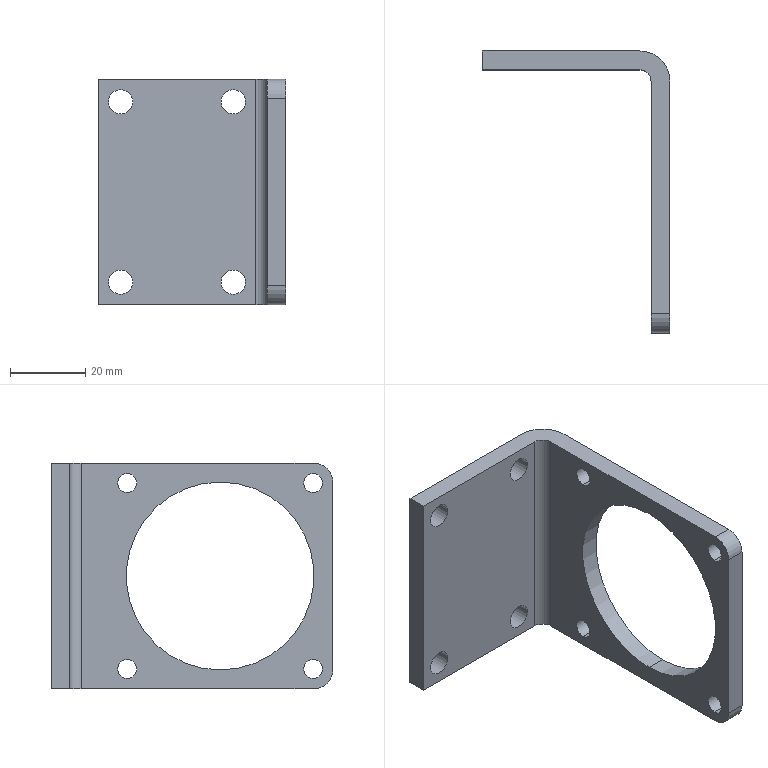Part | STEP file | X77-04012 | 1 solid | 30 faces | box 50 x 75 x 60 mm | volume 24364 mm3 | cylinder 22 | plane 8 | commonest cylinder face diameters 5 x8 6.5 x8 10 x2 50 x2 6 x1 16 x1
STEP:
#1=CARTESIAN_POINT('',(344.189,-36.142,52.249));
#2=VERTEX_POINT('',#1);
#3=CARTESIAN_POINT('',(344.189,-36.142,57.249));
#4=VERTEX_POINT('',#3);
#5=CARTESIAN_POINT('',(344.189,-36.142,54.749));
#6=DIRECTION('',(-1.,0.,0.));
#7=DIRECTION('',(0.,0.,1.));
#8=AXIS2_PLACEMENT_3D('',#5,#6,#7);
#9=CIRCLE('',#8,2.5);
#10=EDGE_CURVE('',#2,#4,#9,.T.);
#11=ORIENTED_EDGE('',*,*,#10,.F.);
#12=CARTESIAN_POINT('',(339.189,-36.142,52.249));
#13=VERTEX_POINT('',#12);
#14=CARTESIAN_POINT('',(339.189,-36.142,52.249));
#15=DIRECTION('',(-1.,0.,0.));
#16=VECTOR('',#15,1000.);
#17=LINE('',#14,#16);
#18=EDGE_CURVE('',#2,#13,#17,.T.);
#19=ORIENTED_EDGE('',*,*,#18,.T.);
#20=CARTESIAN_POINT('',(339.189,-36.142,57.249));
#21=VERTEX_POINT('',#20);
#22=CARTESIAN_POINT('',(339.189,-36.142,54.749));
#23=DIRECTION('',(-1.,0.,0.));
#24=DIRECTION('',(0.,0.,1.));
#25=AXIS2_PLACEMENT_3D('',#22,#23,#24);
#26=CIRCLE('',#25,2.5);
#27=EDGE_CURVE('',#13,#21,#26,.T.);
#28=ORIENTED_EDGE('',*,*,#27,.T.);
#29=CARTESIAN_POINT('',(339.189,-36.142,57.249));
#30=DIRECTION('',(-1.,0.,0.));
#31=VECTOR('',#30,1000.);
#32=LINE('',#29,#31);
#33=EDGE_CURVE('',#4,#21,#32,.T.);
#34=ORIENTED_EDGE('',*,*,#33,.F.);
#35=EDGE_LOOP('',(#11,#19,#28,#34));
#36=FACE_OUTER_BOUND('',#35,.T.);
#37=CARTESIAN_POINT('',(339.189,-36.142,54.749));
#38=DIRECTION('',(-1.,0.,0.));
#39=DIRECTION('',(0.,0.,1.));
#40=AXIS2_PLACEMENT_3D('',#37,#38,#39);
#41=CYLINDRICAL_SURFACE('',#40,2.5);
#42=ADVANCED_FACE('',(#36),#41,.F.);
#43=CARTESIAN_POINT('',(344.189,-36.142,2.751));
#44=VERTEX_POINT('',#43);
#45=CARTESIAN_POINT('',(344.189,-36.142,7.751));
#46=VERTEX_POINT('',#45);
#47=CARTESIAN_POINT('',(344.189,-36.142,5.251));
#48=DIRECTION('',(-1.,0.,0.));
#49=DIRECTION('',(0.,0.,1.));
#50=AXIS2_PLACEMENT_3D('',#47,#48,#49);
#51=CIRCLE('',#50,2.5);
#52=EDGE_CURVE('',#44,#46,#51,.T.);
#53=ORIENTED_EDGE('',*,*,#52,.F.);
#54=CARTESIAN_POINT('',(339.189,-36.142,2.751));
#55=VERTEX_POINT('',#54);
#56=CARTESIAN_POINT('',(339.189,-36.142,2.751));
#57=DIRECTION('',(-1.,0.,0.));
#58=VECTOR('',#57,1000.);
#59=LINE('',#56,#58);
#60=EDGE_CURVE('',#44,#55,#59,.T.);
#61=ORIENTED_EDGE('',*,*,#60,.T.);
#62=CARTESIAN_POINT('',(339.189,-36.142,7.751));
#63=VERTEX_POINT('',#62);
#64=CARTESIAN_POINT('',(339.189,-36.142,5.251));
#65=DIRECTION('',(-1.,0.,0.));
#66=DIRECTION('',(0.,0.,1.));
#67=AXIS2_PLACEMENT_3D('',#64,#65,#66);
#68=CIRCLE('',#67,2.5);
#69=EDGE_CURVE('',#55,#63,#68,.T.);
#70=ORIENTED_EDGE('',*,*,#69,.T.);
#71=CARTESIAN_POINT('',(339.189,-36.142,7.751));
#72=DIRECTION('',(-1.,0.,0.));
#73=VECTOR('',#72,1000.);
#74=LINE('',#71,#73);
#75=EDGE_CURVE('',#46,#63,#74,.T.);
#76=ORIENTED_EDGE('',*,*,#75,.F.);
#77=EDGE_LOOP('',(#53,#61,#70,#76));
#78=FACE_OUTER_BOUND('',#77,.T.);
#79=CARTESIAN_POINT('',(339.189,-36.142,5.251));
#80=DIRECTION('',(-1.,0.,0.));
#81=DIRECTION('',(0.,0.,1.));
#82=AXIS2_PLACEMENT_3D('',#79,#80,#81);
#83=CYLINDRICAL_SURFACE('',#82,2.5);
#84=ADVANCED_FACE('',(#78),#83,.F.);
#85=CARTESIAN_POINT('',(344.189,-85.64,52.249));
#86=VERTEX_POINT('',#85);
#87=CARTESIAN_POINT('',(344.189,-85.64,57.249));
#88=VERTEX_POINT('',#87);
#89=CARTESIAN_POINT('',(344.189,-85.64,54.749));
#90=DIRECTION('',(-1.,0.,0.));
#91=DIRECTION('',(0.,0.,1.));
#92=AXIS2_PLACEMENT_3D('',#89,#90,#91);
#93=CIRCLE('',#92,2.5);
#94=EDGE_CURVE('',#86,#88,#93,.T.);
#95=ORIENTED_EDGE('',*,*,#94,.F.);
#96=CARTESIAN_POINT('',(339.189,-85.64,52.249));
#97=VERTEX_POINT('',#96);
#98=CARTESIAN_POINT('',(339.189,-85.64,52.249));
#99=DIRECTION('',(-1.,0.,0.));
#100=VECTOR('',#99,1000.);
#101=LINE('',#98,#100);
#102=EDGE_CURVE('',#86,#97,#101,.T.);
#103=ORIENTED_EDGE('',*,*,#102,.T.);
#104=CARTESIAN_POINT('',(339.189,-85.64,57.249));
#105=VERTEX_POINT('',#104);
#106=CARTESIAN_POINT('',(339.189,-85.64,54.749));
#107=DIRECTION('',(-1.,0.,0.));
#108=DIRECTION('',(0.,0.,1.));
#109=AXIS2_PLACEMENT_3D('',#106,#107,#108);
#110=CIRCLE('',#109,2.5);
#111=EDGE_CURVE('',#97,#105,#110,.T.);
#112=ORIENTED_EDGE('',*,*,#111,.T.);
#113=CARTESIAN_POINT('',(339.189,-85.64,57.249));
#114=DIRECTION('',(-1.,0.,0.));
#115=VECTOR('',#114,1000.);
#116=LINE('',#113,#115);
#117=EDGE_CURVE('',#88,#105,#116,.T.);
#118=ORIENTED_EDGE('',*,*,#117,.F.);
#119=EDGE_LOOP('',(#95,#103,#112,#118));
#120=FACE_OUTER_BOUND('',#119,.T.);
#121=CARTESIAN_POINT('',(339.189,-85.64,54.749));
#122=DIRECTION('',(-1.,0.,0.));
#123=DIRECTION('',(0.,0.,1.));
#124=AXIS2_PLACEMENT_3D('',#121,#122,#123);
#125=CYLINDRICAL_SURFACE('',#124,2.5);
#126=ADVANCED_FACE('',(#120),#125,.F.);
#127=CARTESIAN_POINT('',(344.189,-85.64,2.751));
#128=VERTEX_POINT('',#127);
#129=CARTESIAN_POINT('',(344.189,-85.64,7.751));
#130=VERTEX_POINT('',#129);
#131=CARTESIAN_POINT('',(344.189,-85.64,5.251));
#132=DIRECTION('',(-1.,0.,0.));
#133=DIRECTION('',(0.,0.,1.));
#134=AXIS2_PLACEMENT_3D('',#131,#132,#133);
#135=CIRCLE('',#134,2.5);
#136=EDGE_CURVE('',#128,#130,#135,.T.);
#137=ORIENTED_EDGE('',*,*,#136,.F.);
#138=CARTESIAN_POINT('',(339.189,-85.64,2.751));
#139=VERTEX_POINT('',#138);
#140=CARTESIAN_POINT('',(339.189,-85.64,2.751));
#141=DIRECTION('',(-1.,0.,0.));
#142=VECTOR('',#141,1000.);
#143=LINE('',#140,#142);
#144=EDGE_CURVE('',#128,#139,#143,.T.);
#145=ORIENTED_EDGE('',*,*,#144,.T.);
#146=CARTESIAN_POINT('',(339.189,-85.64,7.751));
#147=VERTEX_POINT('',#146);
#148=CARTESIAN_POINT('',(339.189,-85.64,5.251));
#149=DIRECTION('',(-1.,0.,0.));
#150=DIRECTION('',(0.,0.,1.));
#151=AXIS2_PLACEMENT_3D('',#148,#149,#150);
#152=CIRCLE('',#151,2.5);
#153=EDGE_CURVE('',#139,#147,#152,.T.);
#154=ORIENTED_EDGE('',*,*,#153,.T.);
#155=CARTESIAN_POINT('',(339.189,-85.64,7.751));
#156=DIRECTION('',(-1.,0.,0.));
#157=VECTOR('',#156,1000.);
#158=LINE('',#155,#157);
#159=EDGE_CURVE('',#130,#147,#158,.T.);
#160=ORIENTED_EDGE('',*,*,#159,.F.);
#161=EDGE_LOOP('',(#137,#145,#154,#160));
#162=FACE_OUTER_BOUND('',#161,.T.);
#163=CARTESIAN_POINT('',(339.189,-85.64,5.251));
#164=DIRECTION('',(-1.,0.,0.));
#165=DIRECTION('',(0.,0.,1.));
#166=AXIS2_PLACEMENT_3D('',#163,#164,#165);
#167=CYLINDRICAL_SURFACE('',#166,2.5);
#168=ADVANCED_FACE('',(#162),#167,.F.);
#169=CARTESIAN_POINT('',(296.939,-15.891,6.));
#170=VERTEX_POINT('',#169);
#171=CARTESIAN_POINT('',(303.439,-15.891,6.));
#172=VERTEX_POINT('',#171);
#173=CARTESIAN_POINT('',(300.189,-15.891,6.));
#174=DIRECTION('',(0.,-1.,0.));
#175=DIRECTION('',(0.,0.,-1.));
#176=AXIS2_PLACEMENT_3D('',#173,#174,#175);
#177=CIRCLE('',#176,3.25);
#178=EDGE_CURVE('',#170,#172,#177,.T.);
#179=ORIENTED_EDGE('',*,*,#178,.F.);
#180=CARTESIAN_POINT('',(296.939,-20.891,6.));
#181=VERTEX_POINT('',#180);
#182=CARTESIAN_POINT('',(296.939,-10.891,6.));
#183=DIRECTION('',(0.,-1.,0.));
#184=VECTOR('',#183,1000.);
#185=LINE('',#182,#184);
#186=EDGE_CURVE('',#170,#181,#185,.T.);
#187=ORIENTED_EDGE('',*,*,#186,.T.);
#188=CARTESIAN_POINT('',(303.439,-20.891,6.));
#189=VERTEX_POINT('',#188);
#190=CARTESIAN_POINT('',(300.189,-20.891,6.));
#191=DIRECTION('',(0.,-1.,0.));
#192=DIRECTION('',(1.,0.,0.));
#193=AXIS2_PLACEMENT_3D('',#190,#191,#192);
#194=CIRCLE('',#193,3.25);
#195=EDGE_CURVE('',#181,#189,#194,.T.);
#196=ORIENTED_EDGE('',*,*,#195,.T.);
#197=CARTESIAN_POINT('',(303.439,-10.891,6.));
#198=DIRECTION('',(0.,-1.,0.));
#199=VECTOR('',#198,1000.);
#200=LINE('',#197,#199);
#201=EDGE_CURVE('',#172,#189,#200,.T.);
#202=ORIENTED_EDGE('',*,*,#201,.F.);
#203=EDGE_LOOP('',(#179,#187,#196,#202));
#204=FACE_OUTER_BOUND('',#203,.T.);
#205=CARTESIAN_POINT('',(300.189,-10.891,6.));
#206=DIRECTION('',(0.,-1.,0.));
#207=DIRECTION('',(1.,0.,0.));
#208=AXIS2_PLACEMENT_3D('',#205,#206,#207);
#209=CYLINDRICAL_SURFACE('',#208,3.25);
#210=ADVANCED_FACE('',(#204),#209,.F.);
#211=CARTESIAN_POINT('',(326.939,-15.891,6.));
#212=VERTEX_POINT('',#211);
#213=CARTESIAN_POINT('',(333.439,-15.891,6.));
#214=VERTEX_POINT('',#213);
#215=CARTESIAN_POINT('',(330.189,-15.891,6.));
#216=DIRECTION('',(0.,-1.,0.));
#217=DIRECTION('',(0.,0.,-1.));
#218=AXIS2_PLACEMENT_3D('',#215,#216,#217);
#219=CIRCLE('',#218,3.25);
#220=EDGE_CURVE('',#212,#214,#219,.T.);
#221=ORIENTED_EDGE('',*,*,#220,.F.);
#222=CARTESIAN_POINT('',(326.939,-20.891,6.));
#223=VERTEX_POINT('',#222);
#224=CARTESIAN_POINT('',(326.939,-10.891,6.));
#225=DIRECTION('',(0.,-1.,0.));
#226=VECTOR('',#225,1000.);
#227=LINE('',#224,#226);
#228=EDGE_CURVE('',#212,#223,#227,.T.);
#229=ORIENTED_EDGE('',*,*,#228,.T.);
#230=CARTESIAN_POINT('',(333.439,-20.891,6.));
#231=VERTEX_POINT('',#230);
#232=CARTESIAN_POINT('',(330.189,-20.891,6.));
#233=DIRECTION('',(0.,-1.,0.));
#234=DIRECTION('',(1.,0.,0.));
#235=AXIS2_PLACEMENT_3D('',#232,#233,#234);
#236=CIRCLE('',#235,3.25);
#237=EDGE_CURVE('',#223,#231,#236,.T.);
#238=ORIENTED_EDGE('',*,*,#237,.T.);
#239=CARTESIAN_POINT('',(333.439,-10.891,6.));
#240=DIRECTION('',(0.,-1.,0.));
#241=VECTOR('',#240,1000.);
#242=LINE('',#239,#241);
#243=EDGE_CURVE('',#214,#231,#242,.T.);
#244=ORIENTED_EDGE('',*,*,#243,.F.);
#245=EDGE_LOOP('',(#221,#229,#238,#244));
#246=FACE_OUTER_BOUND('',#245,.T.);
#247=CARTESIAN_POINT('',(330.189,-10.891,6.));
#248=DIRECTION('',(0.,-1.,0.));
#249=DIRECTION('',(1.,0.,0.));
#250=AXIS2_PLACEMENT_3D('',#247,#248,#249);
#251=CYLINDRICAL_SURFACE('',#250,3.25);
#252=ADVANCED_FACE('',(#246),#251,.F.);
#253=CARTESIAN_POINT('',(326.939,-15.891,54.));
#254=VERTEX_POINT('',#253);
#255=CARTESIAN_POINT('',(333.439,-15.891,54.));
#256=VERTEX_POINT('',#255);
#257=CARTESIAN_POINT('',(330.189,-15.891,54.));
#258=DIRECTION('',(0.,-1.,0.));
#259=DIRECTION('',(0.,0.,-1.));
#260=AXIS2_PLACEMENT_3D('',#257,#258,#259);
#261=CIRCLE('',#260,3.25);
#262=EDGE_CURVE('',#254,#256,#261,.T.);
#263=ORIENTED_EDGE('',*,*,#262,.F.);
#264=CARTESIAN_POINT('',(326.939,-20.891,54.));
#265=VERTEX_POINT('',#264);
#266=CARTESIAN_POINT('',(326.939,-10.891,54.));
#267=DIRECTION('',(0.,-1.,0.));
#268=VECTOR('',#267,1000.);
#269=LINE('',#266,#268);
#270=EDGE_CURVE('',#254,#265,#269,.T.);
#271=ORIENTED_EDGE('',*,*,#270,.T.);
#272=CARTESIAN_POINT('',(333.439,-20.891,54.));
#273=VERTEX_POINT('',#272);
#274=CARTESIAN_POINT('',(330.189,-20.891,54.));
#275=DIRECTION('',(0.,-1.,0.));
#276=DIRECTION('',(1.,0.,0.));
#277=AXIS2_PLACEMENT_3D('',#274,#275,#276);
#278=CIRCLE('',#277,3.25);
#279=EDGE_CURVE('',#265,#273,#278,.T.);
#280=ORIENTED_EDGE('',*,*,#279,.T.);
#281=CARTESIAN_POINT('',(333.439,-10.891,54.));
#282=DIRECTION('',(0.,-1.,0.));
#283=VECTOR('',#282,1000.);
#284=LINE('',#281,#283);
#285=EDGE_CURVE('',#256,#273,#284,.T.);
#286=ORIENTED_EDGE('',*,*,#285,.F.);
#287=EDGE_LOOP('',(#263,#271,#280,#286));
#288=FACE_OUTER_BOUND('',#287,.T.);
#289=CARTESIAN_POINT('',(330.189,-10.891,54.));
#290=DIRECTION('',(0.,-1.,0.));
#291=DIRECTION('',(1.,0.,0.));
#292=AXIS2_PLACEMENT_3D('',#289,#290,#291);
#293=CYLINDRICAL_SURFACE('',#292,3.25);
#294=ADVANCED_FACE('',(#288),#293,.F.);
#295=CARTESIAN_POINT('',(296.939,-15.891,54.));
#296=VERTEX_POINT('',#295);
#297=CARTESIAN_POINT('',(303.439,-15.891,54.));
#298=VERTEX_POINT('',#297);
#299=CARTESIAN_POINT('',(300.189,-15.891,54.));
#300=DIRECTION('',(0.,-1.,0.));
#301=DIRECTION('',(0.,0.,-1.));
#302=AXIS2_PLACEMENT_3D('',#299,#300,#301);
#303=CIRCLE('',#302,3.25);
#304=EDGE_CURVE('',#296,#298,#303,.T.);
#305=ORIENTED_EDGE('',*,*,#304,.F.);
#306=CARTESIAN_POINT('',(296.939,-20.891,54.));
#307=VERTEX_POINT('',#306);
#308=CARTESIAN_POINT('',(296.939,-10.891,54.));
#309=DIRECTION('',(0.,-1.,0.));
#310=VECTOR('',#309,1000.);
#311=LINE('',#308,#310);
#312=EDGE_CURVE('',#296,#307,#311,.T.);
#313=ORIENTED_EDGE('',*,*,#312,.T.);
#314=CARTESIAN_POINT('',(303.439,-20.891,54.));
#315=VERTEX_POINT('',#314);
#316=CARTESIAN_POINT('',(300.189,-20.891,54.));
#317=DIRECTION('',(0.,-1.,0.));
#318=DIRECTION('',(1.,0.,0.));
#319=AXIS2_PLACEMENT_3D('',#316,#317,#318);
#320=CIRCLE('',#319,3.25);
#321=EDGE_CURVE('',#307,#315,#320,.T.);
#322=ORIENTED_EDGE('',*,*,#321,.T.);
#323=CARTESIAN_POINT('',(303.439,-10.891,54.));
#324=DIRECTION('',(0.,-1.,0.));
#325=VECTOR('',#324,1000.);
#326=LINE('',#323,#325);
#327=EDGE_CURVE('',#298,#315,#326,.T.);
#328=ORIENTED_EDGE('',*,*,#327,.F.);
#329=EDGE_LOOP('',(#305,#313,#322,#328));
#330=FACE_OUTER_BOUND('',#329,.T.);
#331=CARTESIAN_POINT('',(300.189,-10.891,54.));
#332=DIRECTION('',(0.,-1.,0.));
#333=DIRECTION('',(1.,0.,0.));
#334=AXIS2_PLACEMENT_3D('',#331,#332,#333);
#335=CYLINDRICAL_SURFACE('',#334,3.25);
#336=ADVANCED_FACE('',(#330),#335,.F.);
#337=CARTESIAN_POINT('',(339.189,-60.891,55.));
#338=VERTEX_POINT('',#337);
#339=CARTESIAN_POINT('',(339.189,-60.891,5.));
#340=VERTEX_POINT('',#339);
#341=CARTESIAN_POINT('',(339.189,-60.891,30.));
#342=DIRECTION('',(1.,0.,0.));
#343=DIRECTION('',(0.,0.,-1.));
#344=AXIS2_PLACEMENT_3D('',#341,#342,#343);
#345=CIRCLE('',#344,25.);
#346=EDGE_CURVE('',#338,#340,#345,.T.);
#347=ORIENTED_EDGE('',*,*,#346,.F.);
#348=CARTESIAN_POINT('',(344.189,-60.891,55.));
#349=VERTEX_POINT('',#348);
#350=CARTESIAN_POINT('',(334.189,-60.891,55.));
#351=DIRECTION('',(1.,0.,0.));
#352=VECTOR('',#351,1000.);
#353=LINE('',#350,#352);
#354=EDGE_CURVE('',#338,#349,#353,.T.);
#355=ORIENTED_EDGE('',*,*,#354,.T.);
#356=CARTESIAN_POINT('',(344.189,-60.891,5.));
#357=VERTEX_POINT('',#356);
#358=CARTESIAN_POINT('',(344.189,-60.891,30.));
#359=DIRECTION('',(1.,0.,0.));
#360=DIRECTION('',(0.,0.,-1.));
#361=AXIS2_PLACEMENT_3D('',#358,#359,#360);
#362=CIRCLE('',#361,25.);
#363=EDGE_CURVE('',#349,#357,#362,.T.);
#364=ORIENTED_EDGE('',*,*,#363,.T.);
#365=CARTESIAN_POINT('',(334.189,-60.891,5.));
#366=DIRECTION('',(1.,0.,0.));
#367=VECTOR('',#366,1000.);
#368=LINE('',#365,#367);
#369=EDGE_CURVE('',#340,#357,#368,.T.);
#370=ORIENTED_EDGE('',*,*,#369,.F.);
#371=EDGE_LOOP('',(#347,#355,#364,#370));
#372=FACE_OUTER_BOUND('',#371,.T.);
#373=CARTESIAN_POINT('',(334.189,-60.891,30.));
#374=DIRECTION('',(1.,0.,0.));
#375=DIRECTION('',(0.,0.,-1.));
#376=AXIS2_PLACEMENT_3D('',#373,#374,#375);
#377=CYLINDRICAL_SURFACE('',#376,25.);
#378=ADVANCED_FACE('',(#372),#377,.F.);
#379=CARTESIAN_POINT('',(339.189,-90.891,55.));
#380=VERTEX_POINT('',#379);
#381=CARTESIAN_POINT('',(339.189,-90.891,5.));
#382=VERTEX_POINT('',#381);
#383=CARTESIAN_POINT('',(339.189,-90.891,60.));
#384=DIRECTION('',(0.,0.,-1.));
#385=VECTOR('',#384,1000.);
#386=LINE('',#383,#385);
#387=EDGE_CURVE('',#380,#382,#386,.T.);
#388=ORIENTED_EDGE('',*,*,#387,.T.);
#389=CARTESIAN_POINT('',(344.189,-90.891,5.));
#390=VERTEX_POINT('',#389);
#391=CARTESIAN_POINT('',(344.189,-90.891,5.));
#392=DIRECTION('',(1.,0.,0.));
#393=VECTOR('',#392,1000.);
#394=LINE('',#391,#393);
#395=EDGE_CURVE('',#382,#390,#394,.T.);
#396=ORIENTED_EDGE('',*,*,#395,.T.);
#397=CARTESIAN_POINT('',(344.189,-90.891,55.));
#398=VERTEX_POINT('',#397);
#399=CARTESIAN_POINT('',(344.189,-90.891,60.));
#400=DIRECTION('',(0.,0.,-1.));
#401=VECTOR('',#400,1000.);
#402=LINE('',#399,#401);
#403=EDGE_CURVE('',#398,#390,#402,.T.);
#404=ORIENTED_EDGE('',*,*,#403,.F.);
#405=CARTESIAN_POINT('',(344.189,-90.891,55.));
#406=DIRECTION('',(-1.,0.,0.));
#407=VECTOR('',#406,1000.);
#408=LINE('',#405,#407);
#409=EDGE_CURVE('',#398,#380,#408,.T.);
#410=ORIENTED_EDGE('',*,*,#409,.T.);
#411=EDGE_LOOP('',(#388,#396,#404,#410));
#412=FACE_OUTER_BOUND('',#411,.T.);
#413=CARTESIAN_POINT('',(344.189,-90.891,60.));
#414=DIRECTION('',(0.,1.,0.));
#415=DIRECTION('',(0.,0.,1.));
#416=AXIS2_PLACEMENT_3D('',#413,#414,#415);
#417=PLANE('',#416);
#418=ADVANCED_FACE('',(#412),#417,.F.);
#419=CARTESIAN_POINT('',(344.189,-36.142,54.749));
#420=DIRECTION('',(-1.,0.,0.));
#421=DIRECTION('',(0.,0.,1.));
#422=AXIS2_PLACEMENT_3D('',#419,#420,#421);
#423=CIRCLE('',#422,2.5);
#424=EDGE_CURVE('',#4,#2,#423,.T.);
#425=ORIENTED_EDGE('',*,*,#424,.T.);
#426=ORIENTED_EDGE('',*,*,#10,.T.);
#427=EDGE_LOOP('',(#425,#426));
#428=FACE_BOUND('',#427,.T.);
#429=CARTESIAN_POINT('',(344.189,-36.142,5.251));
#430=DIRECTION('',(-1.,0.,0.));
#431=DIRECTION('',(0.,0.,1.));
#432=AXIS2_PLACEMENT_3D('',#429,#430,#431);
#433=CIRCLE('',#432,2.5);
#434=EDGE_CURVE('',#46,#44,#433,.T.);
#435=ORIENTED_EDGE('',*,*,#434,.T.);
#436=ORIENTED_EDGE('',*,*,#52,.T.);
#437=EDGE_LOOP('',(#435,#436));
#438=FACE_BOUND('',#437,.T.);
#439=CARTESIAN_POINT('',(344.189,-85.64,54.749));
#440=DIRECTION('',(-1.,0.,0.));
#441=DIRECTION('',(0.,0.,1.));
#442=AXIS2_PLACEMENT_3D('',#439,#440,#441);
#443=CIRCLE('',#442,2.5);
#444=EDGE_CURVE('',#88,#86,#443,.T.);
#445=ORIENTED_EDGE('',*,*,#444,.T.);
#446=ORIENTED_EDGE('',*,*,#94,.T.);
#447=EDGE_LOOP('',(#445,#446));
#448=FACE_BOUND('',#447,.T.);
#449=CARTESIAN_POINT('',(344.189,-85.64,5.251));
#450=DIRECTION('',(-1.,0.,0.));
#451=DIRECTION('',(0.,0.,1.));
#452=AXIS2_PLACEMENT_3D('',#449,#450,#451);
#453=CIRCLE('',#452,2.5);
#454=EDGE_CURVE('',#130,#128,#453,.T.);
#455=ORIENTED_EDGE('',*,*,#454,.T.);
#456=ORIENTED_EDGE('',*,*,#136,.T.);
#457=EDGE_LOOP('',(#455,#456));
#458=FACE_BOUND('',#457,.T.);
#459=CARTESIAN_POINT('',(344.189,-60.891,30.));
#460=DIRECTION('',(1.,0.,0.));
#461=DIRECTION('',(0.,0.,-1.));
#462=AXIS2_PLACEMENT_3D('',#459,#460,#461);
#463=CIRCLE('',#462,25.);
#464=EDGE_CURVE('',#357,#349,#463,.T.);
#465=ORIENTED_EDGE('',*,*,#464,.F.);
#466=ORIENTED_EDGE('',*,*,#363,.F.);
#467=EDGE_LOOP('',(#465,#466));
#468=FACE_BOUND('',#467,.T.);
#469=ORIENTED_EDGE('',*,*,#403,.T.);
#470=CARTESIAN_POINT('',(344.189,-85.891,0.));
#471=VERTEX_POINT('',#470);
#472=CARTESIAN_POINT('',(344.189,-85.891,5.));
#473=DIRECTION('',(1.,0.,0.));
#474=DIRECTION('',(0.,0.,1.));
#475=AXIS2_PLACEMENT_3D('',#472,#473,#474);
#476=CIRCLE('',#475,5.);
#477=EDGE_CURVE('',#390,#471,#476,.T.);
#478=ORIENTED_EDGE('',*,*,#477,.T.);
#479=CARTESIAN_POINT('',(344.189,-23.891,0.));
#480=VERTEX_POINT('',#479);
#481=CARTESIAN_POINT('',(344.189,-23.891,0.));
#482=DIRECTION('',(0.,1.,0.));
#483=VECTOR('',#482,1000.);
#484=LINE('',#481,#483);
#485=EDGE_CURVE('',#471,#480,#484,.T.);
#486=ORIENTED_EDGE('',*,*,#485,.T.);
#487=CARTESIAN_POINT('',(344.189,-23.891,60.));
#488=VERTEX_POINT('',#487);
#489=CARTESIAN_POINT('',(344.189,-23.891,60.));
#490=DIRECTION('',(0.,0.,-1.));
#491=VECTOR('',#490,1000.);
#492=LINE('',#489,#491);
#493=EDGE_CURVE('',#488,#480,#492,.T.);
#494=ORIENTED_EDGE('',*,*,#493,.F.);
#495=CARTESIAN_POINT('',(344.189,-85.891,60.));
#496=VERTEX_POINT('',#495);
#497=CARTESIAN_POINT('',(344.189,-23.891,60.));
#498=DIRECTION('',(0.,1.,0.));
#499=VECTOR('',#498,1000.);
#500=LINE('',#497,#499);
#501=EDGE_CURVE('',#496,#488,#500,.T.);
#502=ORIENTED_EDGE('',*,*,#501,.F.);
#503=CARTESIAN_POINT('',(344.189,-85.891,55.));
#504=DIRECTION('',(1.,0.,0.));
#505=DIRECTION('',(0.,0.,1.));
#506=AXIS2_PLACEMENT_3D('',#503,#504,#505);
#507=CIRCLE('',#506,5.);
#508=EDGE_CURVE('',#496,#398,#507,.T.);
#509=ORIENTED_EDGE('',*,*,#508,.T.);
#510=EDGE_LOOP('',(#469,#478,#486,#494,#502,#509));
#511=FACE_OUTER_BOUND('',#510,.T.);
#512=CARTESIAN_POINT('',(344.189,-23.891,60.));
#513=DIRECTION('',(-1.,0.,0.));
#514=DIRECTION('',(0.,0.,1.));
#515=AXIS2_PLACEMENT_3D('',#512,#513,#514);
#516=PLANE('',#515);
#517=ADVANCED_FACE('',(#428,#438,#448,#458,#468,#511),#516,.F.);
#518=CARTESIAN_POINT('',(336.189,-15.891,0.));
#519=VERTEX_POINT('',#518);
#520=CARTESIAN_POINT('',(336.189,-23.891,0.));
#521=DIRECTION('',(0.,0.,1.));
#522=DIRECTION('',(-1.,0.,0.));
#523=AXIS2_PLACEMENT_3D('',#520,#521,#522);
#524=CIRCLE('',#523,8.);
#525=EDGE_CURVE('',#480,#519,#524,.T.);
#526=ORIENTED_EDGE('',*,*,#525,.T.);
#527=CARTESIAN_POINT('',(336.189,-15.891,60.));
#528=VERTEX_POINT('',#527);
#529=CARTESIAN_POINT('',(336.189,-15.891,60.));
#530=DIRECTION('',(0.,0.,-1.));
#531=VECTOR('',#530,1000.);
#532=LINE('',#529,#531);
#533=EDGE_CURVE('',#528,#519,#532,.T.);
#534=ORIENTED_EDGE('',*,*,#533,.F.);
#535=CARTESIAN_POINT('',(336.189,-23.891,60.));
#536=DIRECTION('',(0.,0.,1.));
#537=DIRECTION('',(-1.,0.,0.));
#538=AXIS2_PLACEMENT_3D('',#535,#536,#537);
#539=CIRCLE('',#538,8.);
#540=EDGE_CURVE('',#488,#528,#539,.T.);
#541=ORIENTED_EDGE('',*,*,#540,.F.);
#542=ORIENTED_EDGE('',*,*,#493,.T.);
#543=EDGE_LOOP('',(#526,#534,#541,#542));
#544=FACE_OUTER_BOUND('',#543,.T.);
#545=CARTESIAN_POINT('',(336.189,-23.891,60.));
#546=DIRECTION('',(0.,0.,-1.));
#547=DIRECTION('',(-1.,0.,0.));
#548=AXIS2_PLACEMENT_3D('',#545,#546,#547);
#549=CYLINDRICAL_SURFACE('',#548,8.);
#550=ADVANCED_FACE('',(#544),#549,.T.);
#551=CARTESIAN_POINT('',(300.189,-15.891,6.));
#552=DIRECTION('',(0.,-1.,0.));
#553=DIRECTION('',(0.,0.,-1.));
#554=AXIS2_PLACEMENT_3D('',#551,#552,#553);
#555=CIRCLE('',#554,3.25);
#556=EDGE_CURVE('',#172,#170,#555,.T.);
#557=ORIENTED_EDGE('',*,*,#556,.T.);
#558=ORIENTED_EDGE('',*,*,#178,.T.);
#559=EDGE_LOOP('',(#557,#558));
#560=FACE_BOUND('',#559,.T.);
#561=CARTESIAN_POINT('',(330.189,-15.891,6.));
#562=DIRECTION('',(0.,-1.,0.));
#563=DIRECTION('',(0.,0.,-1.));
#564=AXIS2_PLACEMENT_3D('',#561,#562,#563);
#565=CIRCLE('',#564,3.25);
#566=EDGE_CURVE('',#214,#212,#565,.T.);
#567=ORIENTED_EDGE('',*,*,#566,.T.);
#568=ORIENTED_EDGE('',*,*,#220,.T.);
#569=EDGE_LOOP('',(#567,#568));
#570=FACE_BOUND('',#569,.T.);
#571=CARTESIAN_POINT('',(330.189,-15.891,54.));
#572=DIRECTION('',(0.,-1.,0.));
#573=DIRECTION('',(0.,0.,-1.));
#574=AXIS2_PLACEMENT_3D('',#571,#572,#573);
#575=CIRCLE('',#574,3.25);
#576=EDGE_CURVE('',#256,#254,#575,.T.);
#577=ORIENTED_EDGE('',*,*,#576,.T.);
#578=ORIENTED_EDGE('',*,*,#262,.T.);
#579=EDGE_LOOP('',(#577,#578));
#580=FACE_BOUND('',#579,.T.);
#581=CARTESIAN_POINT('',(300.189,-15.891,54.));
#582=DIRECTION('',(0.,-1.,0.));
#583=DIRECTION('',(0.,0.,-1.));
#584=AXIS2_PLACEMENT_3D('',#581,#582,#583);
#585=CIRCLE('',#584,3.25);
#586=EDGE_CURVE('',#298,#296,#585,.T.);
#587=ORIENTED_EDGE('',*,*,#586,.T.);
#588=ORIENTED_EDGE('',*,*,#304,.T.);
#589=EDGE_LOOP('',(#587,#588));
#590=FACE_BOUND('',#589,.T.);
#591=CARTESIAN_POINT('',(294.189,-15.891,0.));
#592=VERTEX_POINT('',#591);
#593=CARTESIAN_POINT('',(294.189,-15.891,0.));
#594=DIRECTION('',(-1.,0.,0.));
#595=VECTOR('',#594,1000.);
#596=LINE('',#593,#595);
#597=EDGE_CURVE('',#519,#592,#596,.T.);
#598=ORIENTED_EDGE('',*,*,#597,.T.);
#599=CARTESIAN_POINT('',(294.189,-15.891,60.));
#600=VERTEX_POINT('',#599);
#601=CARTESIAN_POINT('',(294.189,-15.891,60.));
#602=DIRECTION('',(0.,0.,-1.));
#603=VECTOR('',#602,1000.);
#604=LINE('',#601,#603);
#605=EDGE_CURVE('',#600,#592,#604,.T.);
#606=ORIENTED_EDGE('',*,*,#605,.F.);
#607=CARTESIAN_POINT('',(294.189,-15.891,60.));
#608=DIRECTION('',(-1.,0.,0.));
#609=VECTOR('',#608,1000.);
#610=LINE('',#607,#609);
#611=EDGE_CURVE('',#528,#600,#610,.T.);
#612=ORIENTED_EDGE('',*,*,#611,.F.);
#613=ORIENTED_EDGE('',*,*,#533,.T.);
#614=EDGE_LOOP('',(#598,#606,#612,#613));
#615=FACE_OUTER_BOUND('',#614,.T.);
#616=CARTESIAN_POINT('',(294.189,-15.891,60.));
#617=DIRECTION('',(0.,-1.,0.));
#618=DIRECTION('',(0.,0.,-1.));
#619=AXIS2_PLACEMENT_3D('',#616,#617,#618);
#620=PLANE('',#619);
#621=ADVANCED_FACE('',(#560,#570,#580,#590,#615),#620,.F.);
#622=CARTESIAN_POINT('',(294.189,-20.891,0.));
#623=VERTEX_POINT('',#622);
#624=CARTESIAN_POINT('',(294.189,-20.891,0.));
#625=DIRECTION('',(0.,-1.,0.));
#626=VECTOR('',#625,1000.);
#627=LINE('',#624,#626);
#628=EDGE_CURVE('',#592,#623,#627,.T.);
#629=ORIENTED_EDGE('',*,*,#628,.T.);
#630=CARTESIAN_POINT('',(294.189,-20.891,60.));
#631=VERTEX_POINT('',#630);
#632=CARTESIAN_POINT('',(294.189,-20.891,60.));
#633=DIRECTION('',(0.,0.,-1.));
#634=VECTOR('',#633,1000.);
#635=LINE('',#632,#634);
#636=EDGE_CURVE('',#631,#623,#635,.T.);
#637=ORIENTED_EDGE('',*,*,#636,.F.);
#638=CARTESIAN_POINT('',(294.189,-20.891,60.));
#639=DIRECTION('',(0.,-1.,0.));
#640=VECTOR('',#639,1000.);
#641=LINE('',#638,#640);
#642=EDGE_CURVE('',#600,#631,#641,.T.);
#643=ORIENTED_EDGE('',*,*,#642,.F.);
#644=ORIENTED_EDGE('',*,*,#605,.T.);
#645=EDGE_LOOP('',(#629,#637,#643,#644));
#646=FACE_OUTER_BOUND('',#645,.T.);
#647=CARTESIAN_POINT('',(294.189,-20.891,60.));
#648=DIRECTION('',(1.,0.,0.));
#649=DIRECTION('',(0.,0.,-1.));
#650=AXIS2_PLACEMENT_3D('',#647,#648,#649);
#651=PLANE('',#650);
#652=ADVANCED_FACE('',(#646),#651,.F.);
#653=CARTESIAN_POINT('',(300.189,-20.891,6.));
#654=DIRECTION('',(0.,-1.,0.));
#655=DIRECTION('',(1.,0.,0.));
#656=AXIS2_PLACEMENT_3D('',#653,#654,#655);
#657=CIRCLE('',#656,3.25);
#658=EDGE_CURVE('',#189,#181,#657,.T.);
#659=ORIENTED_EDGE('',*,*,#658,.F.);
#660=ORIENTED_EDGE('',*,*,#195,.F.);
#661=EDGE_LOOP('',(#659,#660));
#662=FACE_BOUND('',#661,.T.);
#663=CARTESIAN_POINT('',(330.189,-20.891,6.));
#664=DIRECTION('',(0.,-1.,0.));
#665=DIRECTION('',(1.,0.,0.));
#666=AXIS2_PLACEMENT_3D('',#663,#664,#665);
#667=CIRCLE('',#666,3.25);
#668=EDGE_CURVE('',#231,#223,#667,.T.);
#669=ORIENTED_EDGE('',*,*,#668,.F.);
#670=ORIENTED_EDGE('',*,*,#237,.F.);
#671=EDGE_LOOP('',(#669,#670));
#672=FACE_BOUND('',#671,.T.);
#673=CARTESIAN_POINT('',(330.189,-20.891,54.));
#674=DIRECTION('',(0.,-1.,0.));
#675=DIRECTION('',(1.,0.,0.));
#676=AXIS2_PLACEMENT_3D('',#673,#674,#675);
#677=CIRCLE('',#676,3.25);
#678=EDGE_CURVE('',#273,#265,#677,.T.);
#679=ORIENTED_EDGE('',*,*,#678,.F.);
#680=ORIENTED_EDGE('',*,*,#279,.F.);
#681=EDGE_LOOP('',(#679,#680));
#682=FACE_BOUND('',#681,.T.);
#683=CARTESIAN_POINT('',(300.189,-20.891,54.));
#684=DIRECTION('',(0.,-1.,0.));
#685=DIRECTION('',(1.,0.,0.));
#686=AXIS2_PLACEMENT_3D('',#683,#684,#685);
#687=CIRCLE('',#686,3.25);
#688=EDGE_CURVE('',#315,#307,#687,.T.);
#689=ORIENTED_EDGE('',*,*,#688,.F.);
#690=ORIENTED_EDGE('',*,*,#321,.F.);
#691=EDGE_LOOP('',(#689,#690));
#692=FACE_BOUND('',#691,.T.);
#693=CARTESIAN_POINT('',(336.189,-20.891,0.));
#694=VERTEX_POINT('',#693);
#695=CARTESIAN_POINT('',(336.189,-20.891,0.));
#696=DIRECTION('',(1.,0.,0.));
#697=VECTOR('',#696,1000.);
#698=LINE('',#695,#697);
#699=EDGE_CURVE('',#623,#694,#698,.T.);
#700=ORIENTED_EDGE('',*,*,#699,.T.);
#701=CARTESIAN_POINT('',(336.189,-20.891,60.));
#702=VERTEX_POINT('',#701);
#703=CARTESIAN_POINT('',(336.189,-20.891,60.));
#704=DIRECTION('',(0.,0.,-1.));
#705=VECTOR('',#704,1000.);
#706=LINE('',#703,#705);
#707=EDGE_CURVE('',#702,#694,#706,.T.);
#708=ORIENTED_EDGE('',*,*,#707,.F.);
#709=CARTESIAN_POINT('',(336.189,-20.891,60.));
#710=DIRECTION('',(1.,0.,0.));
#711=VECTOR('',#710,1000.);
#712=LINE('',#709,#711);
#713=EDGE_CURVE('',#631,#702,#712,.T.);
#714=ORIENTED_EDGE('',*,*,#713,.F.);
#715=ORIENTED_EDGE('',*,*,#636,.T.);
#716=EDGE_LOOP('',(#700,#708,#714,#715));
#717=FACE_OUTER_BOUND('',#716,.T.);
#718=CARTESIAN_POINT('',(336.189,-20.891,60.));
#719=DIRECTION('',(0.,1.,0.));
#720=DIRECTION('',(-1.,0.,0.));
#721=AXIS2_PLACEMENT_3D('',#718,#719,#720);
#722=PLANE('',#721);
#723=ADVANCED_FACE('',(#662,#672,#682,#692,#717),#722,.F.);
#724=CARTESIAN_POINT('',(339.189,-23.891,0.));
#725=VERTEX_POINT('',#724);
#726=CARTESIAN_POINT('',(336.189,-23.891,0.));
#727=DIRECTION('',(0.,0.,-1.));
#728=DIRECTION('',(-1.,0.,0.));
#729=AXIS2_PLACEMENT_3D('',#726,#727,#728);
#730=CIRCLE('',#729,3.);
#731=EDGE_CURVE('',#694,#725,#730,.T.);
#732=ORIENTED_EDGE('',*,*,#731,.T.);
#733=CARTESIAN_POINT('',(339.189,-23.891,60.));
#734=VERTEX_POINT('',#733);
#735=CARTESIAN_POINT('',(339.189,-23.891,60.));
#736=DIRECTION('',(0.,0.,-1.));
#737=VECTOR('',#736,1000.);
#738=LINE('',#735,#737);
#739=EDGE_CURVE('',#734,#725,#738,.T.);
#740=ORIENTED_EDGE('',*,*,#739,.F.);
#741=CARTESIAN_POINT('',(336.189,-23.891,60.));
#742=DIRECTION('',(0.,0.,-1.));
#743=DIRECTION('',(-1.,0.,0.));
#744=AXIS2_PLACEMENT_3D('',#741,#742,#743);
#745=CIRCLE('',#744,3.);
#746=EDGE_CURVE('',#702,#734,#745,.T.);
#747=ORIENTED_EDGE('',*,*,#746,.F.);
#748=ORIENTED_EDGE('',*,*,#707,.T.);
#749=EDGE_LOOP('',(#732,#740,#747,#748));
#750=FACE_OUTER_BOUND('',#749,.T.);
#751=CARTESIAN_POINT('',(336.189,-23.891,60.));
#752=DIRECTION('',(0.,0.,-1.));
#753=DIRECTION('',(-1.,0.,0.));
#754=AXIS2_PLACEMENT_3D('',#751,#752,#753);
#755=CYLINDRICAL_SURFACE('',#754,3.);
#756=ADVANCED_FACE('',(#750),#755,.F.);
#757=CARTESIAN_POINT('',(339.189,-36.142,54.749));
#758=DIRECTION('',(-1.,0.,0.));
#759=DIRECTION('',(0.,0.,1.));
#760=AXIS2_PLACEMENT_3D('',#757,#758,#759);
#761=CIRCLE('',#760,2.5);
#762=EDGE_CURVE('',#21,#13,#761,.T.);
#763=ORIENTED_EDGE('',*,*,#762,.F.);
#764=ORIENTED_EDGE('',*,*,#27,.F.);
#765=EDGE_LOOP('',(#763,#764));
#766=FACE_BOUND('',#765,.T.);
#767=CARTESIAN_POINT('',(339.189,-36.142,5.251));
#768=DIRECTION('',(-1.,0.,0.));
#769=DIRECTION('',(0.,0.,1.));
#770=AXIS2_PLACEMENT_3D('',#767,#768,#769);
#771=CIRCLE('',#770,2.5);
#772=EDGE_CURVE('',#63,#55,#771,.T.);
#773=ORIENTED_EDGE('',*,*,#772,.F.);
#774=ORIENTED_EDGE('',*,*,#69,.F.);
#775=EDGE_LOOP('',(#773,#774));
#776=FACE_BOUND('',#775,.T.);
#777=CARTESIAN_POINT('',(339.189,-85.64,54.749));
#778=DIRECTION('',(-1.,0.,0.));
#779=DIRECTION('',(0.,0.,1.));
#780=AXIS2_PLACEMENT_3D('',#777,#778,#779);
#781=CIRCLE('',#780,2.5);
#782=EDGE_CURVE('',#105,#97,#781,.T.);
#783=ORIENTED_EDGE('',*,*,#782,.F.);
#784=ORIENTED_EDGE('',*,*,#111,.F.);
#785=EDGE_LOOP('',(#783,#784));
#786=FACE_BOUND('',#785,.T.);
#787=CARTESIAN_POINT('',(339.189,-85.64,5.251));
#788=DIRECTION('',(-1.,0.,0.));
#789=DIRECTION('',(0.,0.,1.));
#790=AXIS2_PLACEMENT_3D('',#787,#788,#789);
#791=CIRCLE('',#790,2.5);
#792=EDGE_CURVE('',#147,#139,#791,.T.);
#793=ORIENTED_EDGE('',*,*,#792,.F.);
#794=ORIENTED_EDGE('',*,*,#153,.F.);
#795=EDGE_LOOP('',(#793,#794));
#796=FACE_BOUND('',#795,.T.);
#797=CARTESIAN_POINT('',(339.189,-60.891,30.));
#798=DIRECTION('',(1.,0.,0.));
#799=DIRECTION('',(0.,0.,-1.));
#800=AXIS2_PLACEMENT_3D('',#797,#798,#799);
#801=CIRCLE('',#800,25.);
#802=EDGE_CURVE('',#340,#338,#801,.T.);
#803=ORIENTED_EDGE('',*,*,#802,.T.);
#804=ORIENTED_EDGE('',*,*,#346,.T.);
#805=EDGE_LOOP('',(#803,#804));
#806=FACE_BOUND('',#805,.T.);
#807=CARTESIAN_POINT('',(339.189,-85.891,0.));
#808=VERTEX_POINT('',#807);
#809=CARTESIAN_POINT('',(339.189,-90.891,0.));
#810=DIRECTION('',(0.,-1.,0.));
#811=VECTOR('',#810,1000.);
#812=LINE('',#809,#811);
#813=EDGE_CURVE('',#725,#808,#812,.T.);
#814=ORIENTED_EDGE('',*,*,#813,.T.);
#815=CARTESIAN_POINT('',(339.189,-85.891,5.));
#816=DIRECTION('',(-1.,0.,0.));
#817=DIRECTION('',(0.,0.,-1.));
#818=AXIS2_PLACEMENT_3D('',#815,#816,#817);
#819=CIRCLE('',#818,5.);
#820=EDGE_CURVE('',#808,#382,#819,.T.);
#821=ORIENTED_EDGE('',*,*,#820,.T.);
#822=ORIENTED_EDGE('',*,*,#387,.F.);
#823=CARTESIAN_POINT('',(339.189,-85.891,60.));
#824=VERTEX_POINT('',#823);
#825=CARTESIAN_POINT('',(339.189,-85.891,55.));
#826=DIRECTION('',(-1.,0.,0.));
#827=DIRECTION('',(0.,0.,-1.));
#828=AXIS2_PLACEMENT_3D('',#825,#826,#827);
#829=CIRCLE('',#828,5.);
#830=EDGE_CURVE('',#380,#824,#829,.T.);
#831=ORIENTED_EDGE('',*,*,#830,.T.);
#832=CARTESIAN_POINT('',(339.189,-90.891,60.));
#833=DIRECTION('',(0.,-1.,0.));
#834=VECTOR('',#833,1000.);
#835=LINE('',#832,#834);
#836=EDGE_CURVE('',#734,#824,#835,.T.);
#837=ORIENTED_EDGE('',*,*,#836,.F.);
#838=ORIENTED_EDGE('',*,*,#739,.T.);
#839=EDGE_LOOP('',(#814,#821,#822,#831,#837,#838));
#840=FACE_OUTER_BOUND('',#839,.T.);
#841=CARTESIAN_POINT('',(339.189,-90.891,60.));
#842=DIRECTION('',(1.,0.,0.));
#843=DIRECTION('',(0.,0.,-1.));
#844=AXIS2_PLACEMENT_3D('',#841,#842,#843);
#845=PLANE('',#844);
#846=ADVANCED_FACE('',(#766,#776,#786,#796,#806,#840),#845,.F.);
#847=ORIENTED_EDGE('',*,*,#836,.T.);
#848=CARTESIAN_POINT('',(336.189,-85.891,60.));
#849=DIRECTION('',(1.,0.,0.));
#850=VECTOR('',#849,1000.);
#851=LINE('',#848,#850);
#852=EDGE_CURVE('',#824,#496,#851,.T.);
#853=ORIENTED_EDGE('',*,*,#852,.T.);
#854=ORIENTED_EDGE('',*,*,#501,.T.);
#855=ORIENTED_EDGE('',*,*,#540,.T.);
#856=ORIENTED_EDGE('',*,*,#611,.T.);
#857=ORIENTED_EDGE('',*,*,#642,.T.);
#858=ORIENTED_EDGE('',*,*,#713,.T.);
#859=ORIENTED_EDGE('',*,*,#746,.T.);
#860=EDGE_LOOP('',(#847,#853,#854,#855,#856,#857,#858,#859));
#861=FACE_OUTER_BOUND('',#860,.T.);
#862=CARTESIAN_POINT('',(336.189,-23.891,60.));
#863=DIRECTION('',(0.,0.,-1.));
#864=DIRECTION('',(-1.,0.,0.));
#865=AXIS2_PLACEMENT_3D('',#862,#863,#864);
#866=PLANE('',#865);
#867=ADVANCED_FACE('',(#861),#866,.F.);
#868=ORIENTED_EDGE('',*,*,#485,.F.);
#869=CARTESIAN_POINT('',(339.189,-85.891,0.));
#870=DIRECTION('',(-1.,0.,0.));
#871=VECTOR('',#870,1000.);
#872=LINE('',#869,#871);
#873=EDGE_CURVE('',#471,#808,#872,.T.);
#874=ORIENTED_EDGE('',*,*,#873,.T.);
#875=ORIENTED_EDGE('',*,*,#813,.F.);
#876=ORIENTED_EDGE('',*,*,#731,.F.);
#877=ORIENTED_EDGE('',*,*,#699,.F.);
#878=ORIENTED_EDGE('',*,*,#628,.F.);
#879=ORIENTED_EDGE('',*,*,#597,.F.);
#880=ORIENTED_EDGE('',*,*,#525,.F.);
#881=EDGE_LOOP('',(#868,#874,#875,#876,#877,#878,#879,#880));
#882=FACE_OUTER_BOUND('',#881,.T.);
#883=CARTESIAN_POINT('',(336.189,-23.891,0.));
#884=DIRECTION('',(0.,0.,-1.));
#885=DIRECTION('',(-1.,0.,0.));
#886=AXIS2_PLACEMENT_3D('',#883,#884,#885);
#887=PLANE('',#886);
#888=ADVANCED_FACE('',(#882),#887,.T.);
#889=ORIENTED_EDGE('',*,*,#354,.F.);
#890=ORIENTED_EDGE('',*,*,#802,.F.);
#891=ORIENTED_EDGE('',*,*,#369,.T.);
#892=ORIENTED_EDGE('',*,*,#464,.T.);
#893=EDGE_LOOP('',(#889,#890,#891,#892));
#894=FACE_OUTER_BOUND('',#893,.T.);
#895=CARTESIAN_POINT('',(334.189,-60.891,30.));
#896=DIRECTION('',(1.,0.,0.));
#897=DIRECTION('',(0.,0.,-1.));
#898=AXIS2_PLACEMENT_3D('',#895,#896,#897);
#899=CYLINDRICAL_SURFACE('',#898,25.);
#900=ADVANCED_FACE('',(#894),#899,.F.);
#901=ORIENTED_EDGE('',*,*,#820,.F.);
#902=ORIENTED_EDGE('',*,*,#873,.F.);
#903=ORIENTED_EDGE('',*,*,#477,.F.);
#904=ORIENTED_EDGE('',*,*,#395,.F.);
#905=EDGE_LOOP('',(#901,#902,#903,#904));
#906=FACE_OUTER_BOUND('',#905,.T.);
#907=CARTESIAN_POINT('',(344.189,-85.891,5.));
#908=DIRECTION('',(-1.,0.,0.));
#909=DIRECTION('',(0.,0.,1.));
#910=AXIS2_PLACEMENT_3D('',#907,#908,#909);
#911=CYLINDRICAL_SURFACE('',#910,5.);
#912=ADVANCED_FACE('',(#906),#911,.T.);
#913=ORIENTED_EDGE('',*,*,#830,.F.);
#914=ORIENTED_EDGE('',*,*,#409,.F.);
#915=ORIENTED_EDGE('',*,*,#508,.F.);
#916=ORIENTED_EDGE('',*,*,#852,.F.);
#917=EDGE_LOOP('',(#913,#914,#915,#916));
#918=FACE_OUTER_BOUND('',#917,.T.);
#919=CARTESIAN_POINT('',(336.189,-85.891,55.));
#920=DIRECTION('',(1.,0.,0.));
#921=DIRECTION('',(0.,0.,-1.));
#922=AXIS2_PLACEMENT_3D('',#919,#920,#921);
#923=CYLINDRICAL_SURFACE('',#922,5.);
#924=ADVANCED_FACE('',(#918),#923,.T.);
#925=ORIENTED_EDGE('',*,*,#312,.F.);
#926=ORIENTED_EDGE('',*,*,#586,.F.);
#927=ORIENTED_EDGE('',*,*,#327,.T.);
#928=ORIENTED_EDGE('',*,*,#688,.T.);
#929=EDGE_LOOP('',(#925,#926,#927,#928));
#930=FACE_OUTER_BOUND('',#929,.T.);
#931=CARTESIAN_POINT('',(300.189,-10.891,54.));
#932=DIRECTION('',(0.,-1.,0.));
#933=DIRECTION('',(1.,0.,0.));
#934=AXIS2_PLACEMENT_3D('',#931,#932,#933);
#935=CYLINDRICAL_SURFACE('',#934,3.25);
#936=ADVANCED_FACE('',(#930),#935,.F.);
#937=ORIENTED_EDGE('',*,*,#270,.F.);
#938=ORIENTED_EDGE('',*,*,#576,.F.);
#939=ORIENTED_EDGE('',*,*,#285,.T.);
#940=ORIENTED_EDGE('',*,*,#678,.T.);
#941=EDGE_LOOP('',(#937,#938,#939,#940));
#942=FACE_OUTER_BOUND('',#941,.T.);
#943=CARTESIAN_POINT('',(330.189,-10.891,54.));
#944=DIRECTION('',(0.,-1.,0.));
#945=DIRECTION('',(1.,0.,0.));
#946=AXIS2_PLACEMENT_3D('',#943,#944,#945);
#947=CYLINDRICAL_SURFACE('',#946,3.25);
#948=ADVANCED_FACE('',(#942),#947,.F.);
#949=ORIENTED_EDGE('',*,*,#228,.F.);
#950=ORIENTED_EDGE('',*,*,#566,.F.);
#951=ORIENTED_EDGE('',*,*,#243,.T.);
#952=ORIENTED_EDGE('',*,*,#668,.T.);
#953=EDGE_LOOP('',(#949,#950,#951,#952));
#954=FACE_OUTER_BOUND('',#953,.T.);
#955=CARTESIAN_POINT('',(330.189,-10.891,6.));
#956=DIRECTION('',(0.,-1.,0.));
#957=DIRECTION('',(1.,0.,0.));
#958=AXIS2_PLACEMENT_3D('',#955,#956,#957);
#959=CYLINDRICAL_SURFACE('',#958,3.25);
#960=ADVANCED_FACE('',(#954),#959,.F.);
#961=ORIENTED_EDGE('',*,*,#186,.F.);
#962=ORIENTED_EDGE('',*,*,#556,.F.);
#963=ORIENTED_EDGE('',*,*,#201,.T.);
#964=ORIENTED_EDGE('',*,*,#658,.T.);
#965=EDGE_LOOP('',(#961,#962,#963,#964));
#966=FACE_OUTER_BOUND('',#965,.T.);
#967=CARTESIAN_POINT('',(300.189,-10.891,6.));
#968=DIRECTION('',(0.,-1.,0.));
#969=DIRECTION('',(1.,0.,0.));
#970=AXIS2_PLACEMENT_3D('',#967,#968,#969);
#971=CYLINDRICAL_SURFACE('',#970,3.25);
#972=ADVANCED_FACE('',(#966),#971,.F.);
#973=ORIENTED_EDGE('',*,*,#144,.F.);
#974=ORIENTED_EDGE('',*,*,#454,.F.);
#975=ORIENTED_EDGE('',*,*,#159,.T.);
#976=ORIENTED_EDGE('',*,*,#792,.T.);
#977=EDGE_LOOP('',(#973,#974,#975,#976));
#978=FACE_OUTER_BOUND('',#977,.T.);
#979=CARTESIAN_POINT('',(339.189,-85.64,5.251));
#980=DIRECTION('',(-1.,0.,0.));
#981=DIRECTION('',(0.,0.,1.));
#982=AXIS2_PLACEMENT_3D('',#979,#980,#981);
#983=CYLINDRICAL_SURFACE('',#982,2.5);
#984=ADVANCED_FACE('',(#978),#983,.F.);
#985=ORIENTED_EDGE('',*,*,#102,.F.);
#986=ORIENTED_EDGE('',*,*,#444,.F.);
#987=ORIENTED_EDGE('',*,*,#117,.T.);
#988=ORIENTED_EDGE('',*,*,#782,.T.);
#989=EDGE_LOOP('',(#985,#986,#987,#988));
#990=FACE_OUTER_BOUND('',#989,.T.);
#991=CARTESIAN_POINT('',(339.189,-85.64,54.749));
#992=DIRECTION('',(-1.,0.,0.));
#993=DIRECTION('',(0.,0.,1.));
#994=AXIS2_PLACEMENT_3D('',#991,#992,#993);
#995=CYLINDRICAL_SURFACE('',#994,2.5);
#996=ADVANCED_FACE('',(#990),#995,.F.);
#997=ORIENTED_EDGE('',*,*,#60,.F.);
#998=ORIENTED_EDGE('',*,*,#434,.F.);
#999=ORIENTED_EDGE('',*,*,#75,.T.);
#1000=ORIENTED_EDGE('',*,*,#772,.T.);
#1001=EDGE_LOOP('',(#997,#998,#999,#1000));
#1002=FACE_OUTER_BOUND('',#1001,.T.);
#1003=CARTESIAN_POINT('',(339.189,-36.142,5.251));
#1004=DIRECTION('',(-1.,0.,0.));
#1005=DIRECTION('',(0.,0.,1.));
#1006=AXIS2_PLACEMENT_3D('',#1003,#1004,#1005);
#1007=CYLINDRICAL_SURFACE('',#1006,2.5);
#1008=ADVANCED_FACE('',(#1002),#1007,.F.);
#1009=ORIENTED_EDGE('',*,*,#18,.F.);
#1010=ORIENTED_EDGE('',*,*,#424,.F.);
#1011=ORIENTED_EDGE('',*,*,#33,.T.);
#1012=ORIENTED_EDGE('',*,*,#762,.T.);
#1013=EDGE_LOOP('',(#1009,#1010,#1011,#1012));
#1014=FACE_OUTER_BOUND('',#1013,.T.);
#1015=CARTESIAN_POINT('',(339.189,-36.142,54.749));
#1016=DIRECTION('',(-1.,0.,0.));
#1017=DIRECTION('',(0.,0.,1.));
#1018=AXIS2_PLACEMENT_3D('',#1015,#1016,#1017);
#1019=CYLINDRICAL_SURFACE('',#1018,2.5);
#1020=ADVANCED_FACE('',(#1014),#1019,.F.);
#1021=CLOSED_SHELL('',(#42,#84,#126,#168,#210,#252,#294,#336,#378,#418,#517,#550,#621,#652,#723,#756,#846,#867,#888,#900,#912,#924,#936,#948,#960,#972,#984,#996,#1008,#1020));
#1022=MANIFOLD_SOLID_BREP('',#1021);
#1023=CARTESIAN_POINT('',(0.,0.,0.));
#1024=DIRECTION('',(0.,0.,1.));
#1025=DIRECTION('',(1.,0.,0.));
#1026=AXIS2_PLACEMENT_3D('',#1023,#1024,#1025);
#1027=(LENGTH_UNIT()NAMED_UNIT(*)SI_UNIT(.MILLI.,.METRE.));
#1028=UNCERTAINTY_MEASURE_WITH_UNIT(LENGTH_MEASURE(0.00001),#1027,'','');
#1029=(NAMED_UNIT(*)PLANE_ANGLE_UNIT()SI_UNIT($,.RADIAN.));
#1030=(NAMED_UNIT(*)SI_UNIT($,.STERADIAN.)SOLID_ANGLE_UNIT());
#1031=(GEOMETRIC_REPRESENTATION_CONTEXT(3)GLOBAL_UNCERTAINTY_ASSIGNED_CONTEXT((#1028))GLOBAL_UNIT_ASSIGNED_CONTEXT((#1027,#1029,#1030))REPRESENTATION_CONTEXT('',''));
#1032=ADVANCED_BREP_SHAPE_REPRESENTATION('',(#1022,#1026),#1031);